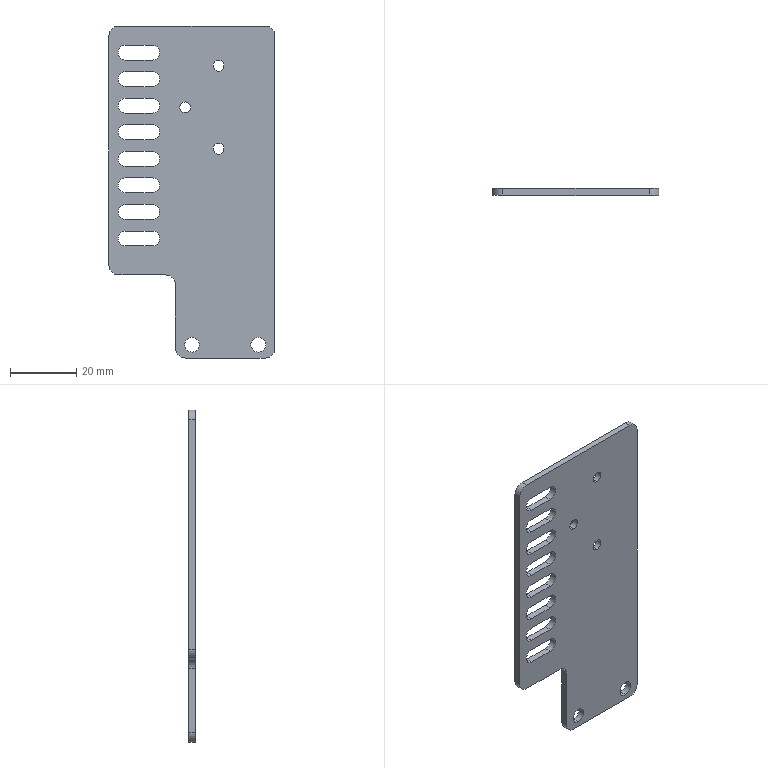Part | NX | features BREP 1 | 1 solid | 56 faces | box 50 x 2 x 100 mm | volume 8039 mm3 | cylinder 32 | plane 24 | commonest cylinder face diameters 4.5 x20 3.3 x6 6 x6